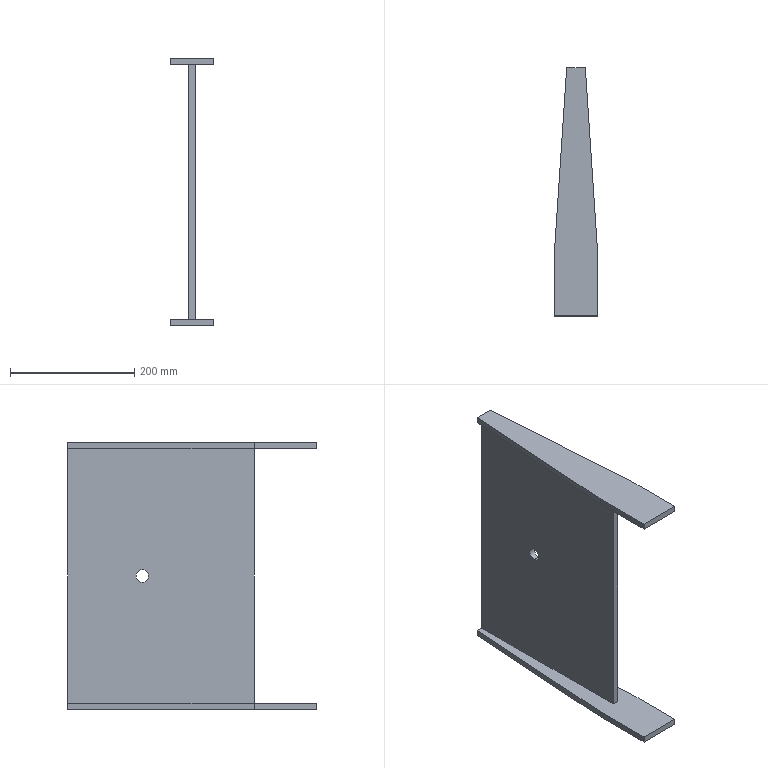Part | STEP file | 3 solids | 24 faces | box 70 x 400 x 430 mm | volume 1666858 mm3 | plane 22 | cylinder 2 | commonest cylinder face diameters 20 x2